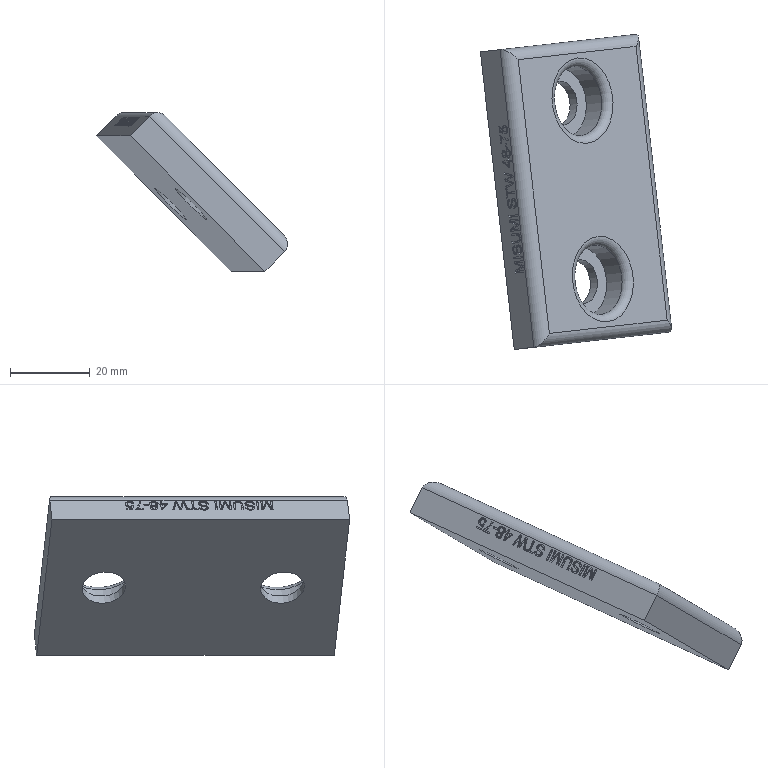Part | NX | features solid 2 | 1 solid | 149 faces | box 47.914 x 78.929 x 39.77 mm | volume 31346 mm3 | plane 107 | spline 32 | cylinder 8 | torus 2 | commonest cylinder face diameters 6 x4 11 x2 17.5 x2